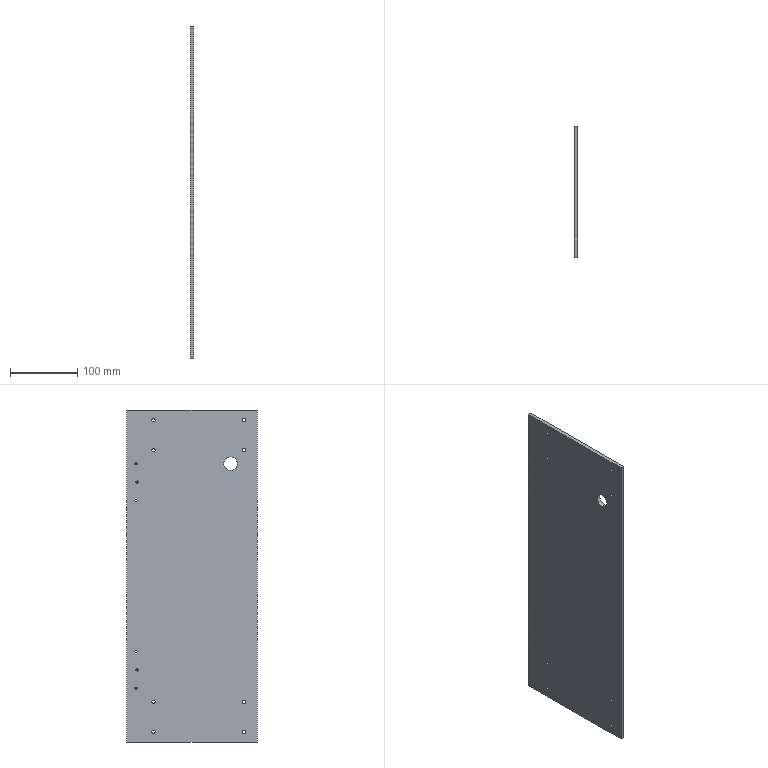Part | STEP file | 09-09 Outer side plate 2 | 1 solid | 36 faces | box 5 x 195 x 495 mm | volume 480012 mm3 | cylinder 30 | plane 6 | commonest cylinder face diameters 5 x16 3.3 x12 20 x2